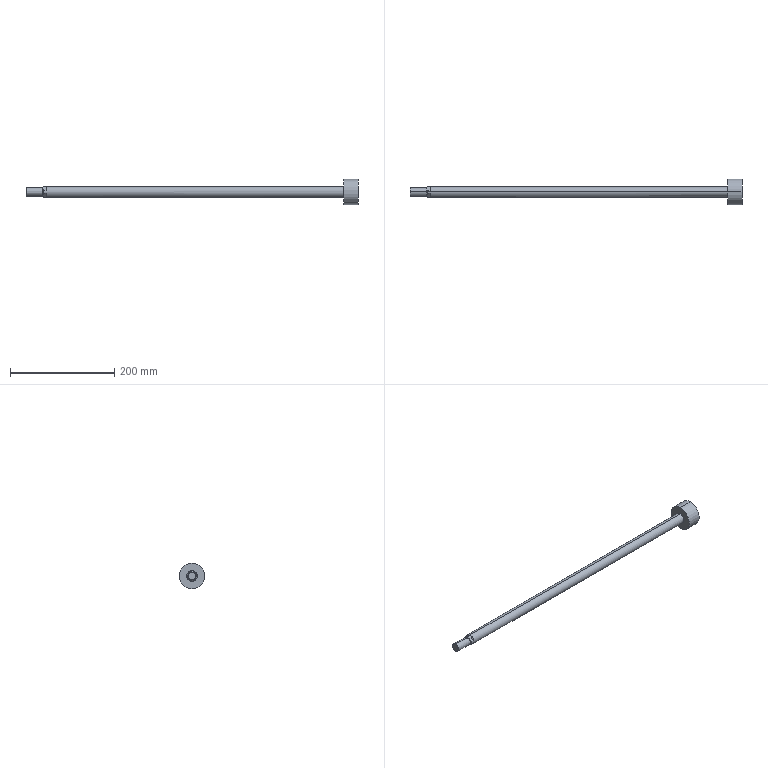Part | NX | features BREP 1 | 1 solid | 21 faces | box 635.5 x 49.1 x 49.1 mm | volume 238288 mm3 | plane 11 | cylinder 6 | cone 4 | commonest cylinder face diameters 16 x2 20 x2 49.1 x2
STEP:
#1=CARTESIAN_POINT('',(539.5,0.,10.));
#2=VERTEX_POINT('',#1);
#3=CARTESIAN_POINT('',(539.5,0.,-10.));
#4=VERTEX_POINT('',#3);
#5=CARTESIAN_POINT('',(539.5,0.,0.));
#6=DIRECTION('',(-1.,0.,0.));
#7=DIRECTION('',(0.,0.,1.));
#8=AXIS2_PLACEMENT_3D('',#5,#6,#7);
#9=CIRCLE('',#8,10.);
#10=EDGE_CURVE('',#2,#4,#9,.T.);
#11=ORIENTED_EDGE('',*,*,#10,.T.);
#12=CARTESIAN_POINT('',(-35.,0.,-10.));
#13=VERTEX_POINT('',#12);
#14=CARTESIAN_POINT('',(566.5,0.,-10.));
#15=DIRECTION('',(-1.,0.,0.));
#16=VECTOR('',#15,1000.);
#17=LINE('',#14,#16);
#18=EDGE_CURVE('',#13,#4,#17,.F.);
#19=ORIENTED_EDGE('',*,*,#18,.F.);
#20=CARTESIAN_POINT('',(-35.,2.285,-9.735));
#21=VERTEX_POINT('',#20);
#22=CARTESIAN_POINT('',(-35.,0.,0.));
#23=DIRECTION('',(1.,0.,0.));
#24=DIRECTION('',(0.,0.,1.));
#25=AXIS2_PLACEMENT_3D('',#22,#23,#24);
#26=CIRCLE('',#25,10.);
#27=EDGE_CURVE('',#13,#21,#26,.T.);
#28=ORIENTED_EDGE('',*,*,#27,.T.);
#29=CARTESIAN_POINT('',(-30.5,2.285,-9.735));
#30=VERTEX_POINT('',#29);
#31=CARTESIAN_POINT('',(566.5,2.285,-9.735));
#32=DIRECTION('',(1.,0.,0.));
#33=VECTOR('',#32,1000.);
#34=LINE('',#31,#33);
#35=EDGE_CURVE('',#21,#30,#34,.T.);
#36=ORIENTED_EDGE('',*,*,#35,.T.);
#37=CARTESIAN_POINT('',(-30.5,9.735,-2.285));
#38=VERTEX_POINT('',#37);
#39=CARTESIAN_POINT('',(-30.5,2.285,-9.735));
#40=CARTESIAN_POINT('',(-28.444,6.084,-8.844));
#41=CARTESIAN_POINT('',(-28.444,8.844,-6.084));
#42=CARTESIAN_POINT('',(-30.5,9.735,-2.285));
#43=(BOUNDED_CURVE()B_SPLINE_CURVE(3,(#39,#40,#41,#42),.UNSPECIFIED.,.F.,.F.)B_SPLINE_CURVE_WITH_KNOTS((4,4),(2.587,3.696),.UNSPECIFIED.)CURVE()GEOMETRIC_REPRESENTATION_ITEM()RATIONAL_B_SPLINE_CURVE((1.,0.9,0.9,1.))REPRESENTATION_ITEM(''));
#44=EDGE_CURVE('',#30,#38,#43,.T.);
#45=ORIENTED_EDGE('',*,*,#44,.T.);
#46=CARTESIAN_POINT('',(-35.,9.735,-2.285));
#47=VERTEX_POINT('',#46);
#48=CARTESIAN_POINT('',(566.5,9.735,-2.285));
#49=DIRECTION('',(-1.,0.,0.));
#50=VECTOR('',#49,1000.);
#51=LINE('',#48,#50);
#52=EDGE_CURVE('',#38,#47,#51,.T.);
#53=ORIENTED_EDGE('',*,*,#52,.T.);
#54=CARTESIAN_POINT('',(-35.,9.735,2.285));
#55=VERTEX_POINT('',#54);
#56=CARTESIAN_POINT('',(-35.,0.,0.));
#57=DIRECTION('',(1.,0.,0.));
#58=DIRECTION('',(0.,0.,1.));
#59=AXIS2_PLACEMENT_3D('',#56,#57,#58);
#60=CIRCLE('',#59,10.);
#61=EDGE_CURVE('',#47,#55,#60,.T.);
#62=ORIENTED_EDGE('',*,*,#61,.T.);
#63=CARTESIAN_POINT('',(-30.5,9.735,2.285));
#64=VERTEX_POINT('',#63);
#65=CARTESIAN_POINT('',(566.5,9.735,2.285));
#66=DIRECTION('',(1.,0.,0.));
#67=VECTOR('',#66,1000.);
#68=LINE('',#65,#67);
#69=EDGE_CURVE('',#55,#64,#68,.T.);
#70=ORIENTED_EDGE('',*,*,#69,.T.);
#71=CARTESIAN_POINT('',(-30.5,2.285,9.735));
#72=VERTEX_POINT('',#71);
#73=CARTESIAN_POINT('',(-30.5,9.735,2.285));
#74=CARTESIAN_POINT('',(-28.444,8.844,6.084));
#75=CARTESIAN_POINT('',(-28.444,6.084,8.844));
#76=CARTESIAN_POINT('',(-30.5,2.285,9.735));
#77=(BOUNDED_CURVE()B_SPLINE_CURVE(3,(#73,#74,#75,#76),.UNSPECIFIED.,.F.,.F.)B_SPLINE_CURVE_WITH_KNOTS((4,4),(2.587,3.696),.UNSPECIFIED.)CURVE()GEOMETRIC_REPRESENTATION_ITEM()RATIONAL_B_SPLINE_CURVE((1.,0.9,0.9,1.))REPRESENTATION_ITEM(''));
#78=EDGE_CURVE('',#64,#72,#77,.T.);
#79=ORIENTED_EDGE('',*,*,#78,.T.);
#80=CARTESIAN_POINT('',(-35.,2.285,9.735));
#81=VERTEX_POINT('',#80);
#82=CARTESIAN_POINT('',(566.5,2.285,9.735));
#83=DIRECTION('',(-1.,0.,0.));
#84=VECTOR('',#83,1000.);
#85=LINE('',#82,#84);
#86=EDGE_CURVE('',#72,#81,#85,.T.);
#87=ORIENTED_EDGE('',*,*,#86,.T.);
#88=CARTESIAN_POINT('',(-35.,0.,10.));
#89=VERTEX_POINT('',#88);
#90=CARTESIAN_POINT('',(-35.,0.,0.));
#91=DIRECTION('',(1.,0.,0.));
#92=DIRECTION('',(0.,0.,1.));
#93=AXIS2_PLACEMENT_3D('',#90,#91,#92);
#94=CIRCLE('',#93,10.);
#95=EDGE_CURVE('',#81,#89,#94,.T.);
#96=ORIENTED_EDGE('',*,*,#95,.T.);
#97=CARTESIAN_POINT('',(566.5,0.,10.));
#98=DIRECTION('',(-1.,0.,0.));
#99=VECTOR('',#98,1000.);
#100=LINE('',#97,#99);
#101=EDGE_CURVE('',#89,#2,#100,.F.);
#102=ORIENTED_EDGE('',*,*,#101,.T.);
#103=EDGE_LOOP('',(#11,#19,#28,#36,#45,#53,#62,#70,#79,#87,#96,#102));
#104=FACE_BOUND('',#103,.T.);
#105=CARTESIAN_POINT('',(566.5,0.,0.));
#106=DIRECTION('',(-1.,0.,0.));
#107=DIRECTION('',(0.,0.,1.));
#108=AXIS2_PLACEMENT_3D('',#105,#106,#107);
#109=CYLINDRICAL_SURFACE('',#108,10.);
#110=ADVANCED_FACE('',(#104),#109,.T.);
#111=CARTESIAN_POINT('',(-37.,0.,-8.));
#112=VERTEX_POINT('',#111);
#113=CARTESIAN_POINT('',(-37.,0.,8.));
#114=VERTEX_POINT('',#113);
#115=CARTESIAN_POINT('',(-37.,0.,0.));
#116=DIRECTION('',(1.,0.,0.));
#117=DIRECTION('',(0.,0.,-1.));
#118=AXIS2_PLACEMENT_3D('',#115,#116,#117);
#119=CIRCLE('',#118,8.);
#120=EDGE_CURVE('',#112,#114,#119,.T.);
#121=ORIENTED_EDGE('',*,*,#120,.T.);
#122=CARTESIAN_POINT('',(-35.,0.,10.));
#123=DIRECTION('',(0.7071,0.,0.7071));
#124=VECTOR('',#123,1000.);
#125=LINE('',#122,#124);
#126=EDGE_CURVE('',#114,#89,#125,.T.);
#127=ORIENTED_EDGE('',*,*,#126,.T.);
#128=ORIENTED_EDGE('',*,*,#95,.F.);
#129=CARTESIAN_POINT('',(-35.,9.735,2.285));
#130=CARTESIAN_POINT('',(-35.469,9.106,2.915));
#131=CARTESIAN_POINT('',(-35.982,8.278,3.743));
#132=CARTESIAN_POINT('',(-36.426,6.984,5.037));
#133=CARTESIAN_POINT('',(-36.537,6.009,6.011));
#134=CARTESIAN_POINT('',(-36.427,5.037,6.984));
#135=CARTESIAN_POINT('',(-36.089,4.056,7.965));
#136=CARTESIAN_POINT('',(-35.654,3.227,8.794));
#137=CARTESIAN_POINT('',(-35.236,2.602,9.419));
#138=CARTESIAN_POINT('',(-35.,2.285,9.735));
#139=B_SPLINE_CURVE_WITH_KNOTS('',3,(#129,#130,#131,#132,#133,#134,#135,#136,#137,#138),.UNSPECIFIED.,.F.,.F.,(4,1,1,1,1,1,1,4),(0.,0.25,0.375,0.5,0.625,0.75,0.875,1.),.UNSPECIFIED.);
#140=EDGE_CURVE('',#81,#55,#139,.F.);
#141=ORIENTED_EDGE('',*,*,#140,.T.);
#142=ORIENTED_EDGE('',*,*,#61,.F.);
#143=CARTESIAN_POINT('',(-35.,2.285,-9.735));
#144=CARTESIAN_POINT('',(-35.469,2.915,-9.106));
#145=CARTESIAN_POINT('',(-35.982,3.743,-8.278));
#146=CARTESIAN_POINT('',(-36.426,5.037,-6.984));
#147=CARTESIAN_POINT('',(-36.537,6.011,-6.009));
#148=CARTESIAN_POINT('',(-36.427,6.984,-5.037));
#149=CARTESIAN_POINT('',(-36.089,7.965,-4.056));
#150=CARTESIAN_POINT('',(-35.654,8.794,-3.227));
#151=CARTESIAN_POINT('',(-35.236,9.419,-2.602));
#152=CARTESIAN_POINT('',(-35.,9.735,-2.285));
#153=B_SPLINE_CURVE_WITH_KNOTS('',3,(#143,#144,#145,#146,#147,#148,#149,#150,#151,#152),.UNSPECIFIED.,.F.,.F.,(4,1,1,1,1,1,1,4),(0.,0.25,0.375,0.5,0.625,0.75,0.875,1.),.UNSPECIFIED.);
#154=EDGE_CURVE('',#47,#21,#153,.F.);
#155=ORIENTED_EDGE('',*,*,#154,.T.);
#156=ORIENTED_EDGE('',*,*,#27,.F.);
#157=CARTESIAN_POINT('',(-35.,0.,-10.));
#158=DIRECTION('',(0.7071,0.,-0.7071));
#159=VECTOR('',#158,1000.);
#160=LINE('',#157,#159);
#161=EDGE_CURVE('',#112,#13,#160,.T.);
#162=ORIENTED_EDGE('',*,*,#161,.F.);
#163=EDGE_LOOP('',(#121,#127,#128,#141,#142,#155,#156,#162));
#164=FACE_BOUND('',#163,.T.);
#165=CARTESIAN_POINT('',(-35.,0.,0.));
#166=DIRECTION('',(1.,0.,0.));
#167=DIRECTION('',(0.,0.,-1.));
#168=AXIS2_PLACEMENT_3D('',#165,#166,#167);
#169=CONICAL_SURFACE('',#168,10.,0.7854);
#170=ADVANCED_FACE('',(#164),#169,.T.);
#171=ORIENTED_EDGE('',*,*,#120,.F.);
#172=CARTESIAN_POINT('',(-68.08,0.,-8.));
#173=VERTEX_POINT('',#172);
#174=CARTESIAN_POINT('',(566.5,0.,-8.));
#175=DIRECTION('',(-1.,0.,0.));
#176=VECTOR('',#175,1000.);
#177=LINE('',#174,#176);
#178=EDGE_CURVE('',#173,#112,#177,.F.);
#179=ORIENTED_EDGE('',*,*,#178,.F.);
#180=CARTESIAN_POINT('',(-68.08,0.,8.));
#181=VERTEX_POINT('',#180);
#182=CARTESIAN_POINT('',(-68.08,0.,0.));
#183=DIRECTION('',(1.,0.,0.));
#184=DIRECTION('',(0.,0.,1.));
#185=AXIS2_PLACEMENT_3D('',#182,#183,#184);
#186=CIRCLE('',#185,8.);
#187=EDGE_CURVE('',#173,#181,#186,.T.);
#188=ORIENTED_EDGE('',*,*,#187,.T.);
#189=CARTESIAN_POINT('',(566.5,0.,8.));
#190=DIRECTION('',(-1.,0.,0.));
#191=VECTOR('',#190,1000.);
#192=LINE('',#189,#191);
#193=EDGE_CURVE('',#181,#114,#192,.F.);
#194=ORIENTED_EDGE('',*,*,#193,.T.);
#195=EDGE_LOOP('',(#171,#179,#188,#194));
#196=FACE_BOUND('',#195,.T.);
#197=CARTESIAN_POINT('',(566.5,0.,0.));
#198=DIRECTION('',(-1.,0.,0.));
#199=DIRECTION('',(0.,0.,1.));
#200=AXIS2_PLACEMENT_3D('',#197,#198,#199);
#201=CYLINDRICAL_SURFACE('',#200,8.);
#202=ADVANCED_FACE('',(#196),#201,.T.);
#203=CARTESIAN_POINT('',(566.5,0.,24.55));
#204=VERTEX_POINT('',#203);
#205=CARTESIAN_POINT('',(566.5,0.,-24.55));
#206=VERTEX_POINT('',#205);
#207=CARTESIAN_POINT('',(566.5,0.,0.));
#208=DIRECTION('',(-1.,0.,0.));
#209=DIRECTION('',(0.,0.,1.));
#210=AXIS2_PLACEMENT_3D('',#207,#208,#209);
#211=CIRCLE('',#210,24.55);
#212=EDGE_CURVE('',#204,#206,#211,.T.);
#213=ORIENTED_EDGE('',*,*,#212,.T.);
#214=CARTESIAN_POINT('',(539.5,0.,-24.55));
#215=VERTEX_POINT('',#214);
#216=CARTESIAN_POINT('',(566.5,0.,-24.55));
#217=DIRECTION('',(-1.,0.,0.));
#218=VECTOR('',#217,1000.);
#219=LINE('',#216,#218);
#220=EDGE_CURVE('',#215,#206,#219,.F.);
#221=ORIENTED_EDGE('',*,*,#220,.F.);
#222=CARTESIAN_POINT('',(539.5,0.,24.55));
#223=VERTEX_POINT('',#222);
#224=CARTESIAN_POINT('',(539.5,0.,0.));
#225=DIRECTION('',(1.,0.,0.));
#226=DIRECTION('',(0.,0.,1.));
#227=AXIS2_PLACEMENT_3D('',#224,#225,#226);
#228=CIRCLE('',#227,24.55);
#229=EDGE_CURVE('',#215,#223,#228,.T.);
#230=ORIENTED_EDGE('',*,*,#229,.T.);
#231=CARTESIAN_POINT('',(566.5,0.,24.55));
#232=DIRECTION('',(-1.,0.,0.));
#233=VECTOR('',#232,1000.);
#234=LINE('',#231,#233);
#235=EDGE_CURVE('',#223,#204,#234,.F.);
#236=ORIENTED_EDGE('',*,*,#235,.T.);
#237=EDGE_LOOP('',(#213,#221,#230,#236));
#238=FACE_BOUND('',#237,.T.);
#239=CARTESIAN_POINT('',(566.5,0.,0.));
#240=DIRECTION('',(-1.,0.,0.));
#241=DIRECTION('',(0.,0.,1.));
#242=AXIS2_PLACEMENT_3D('',#239,#240,#241);
#243=CYLINDRICAL_SURFACE('',#242,24.55);
#244=ADVANCED_FACE('',(#238),#243,.T.);
#245=CARTESIAN_POINT('',(-69.,0.,-7.08));
#246=VERTEX_POINT('',#245);
#247=CARTESIAN_POINT('',(-69.,0.,7.08));
#248=VERTEX_POINT('',#247);
#249=CARTESIAN_POINT('',(-69.,0.,0.));
#250=DIRECTION('',(1.,0.,0.));
#251=DIRECTION('',(0.,0.,-1.));
#252=AXIS2_PLACEMENT_3D('',#249,#250,#251);
#253=CIRCLE('',#252,7.08);
#254=EDGE_CURVE('',#246,#248,#253,.T.);
#255=ORIENTED_EDGE('',*,*,#254,.T.);
#256=CARTESIAN_POINT('',(-68.08,0.,8.));
#257=DIRECTION('',(0.7071,0.,0.7071));
#258=VECTOR('',#257,1000.);
#259=LINE('',#256,#258);
#260=EDGE_CURVE('',#248,#181,#259,.T.);
#261=ORIENTED_EDGE('',*,*,#260,.T.);
#262=ORIENTED_EDGE('',*,*,#187,.F.);
#263=CARTESIAN_POINT('',(-68.08,0.,-8.));
#264=DIRECTION('',(0.7071,0.,-0.7071));
#265=VECTOR('',#264,1000.);
#266=LINE('',#263,#265);
#267=EDGE_CURVE('',#246,#173,#266,.T.);
#268=ORIENTED_EDGE('',*,*,#267,.F.);
#269=EDGE_LOOP('',(#255,#261,#262,#268));
#270=FACE_BOUND('',#269,.T.);
#271=CARTESIAN_POINT('',(-68.08,0.,0.));
#272=DIRECTION('',(1.,0.,0.));
#273=DIRECTION('',(0.,0.,-1.));
#274=AXIS2_PLACEMENT_3D('',#271,#272,#273);
#275=CONICAL_SURFACE('',#274,8.,0.7854);
#276=ADVANCED_FACE('',(#270),#275,.T.);
#277=ORIENTED_EDGE('',*,*,#18,.T.);
#278=CARTESIAN_POINT('',(539.5,0.,0.));
#279=DIRECTION('',(-1.,0.,0.));
#280=DIRECTION('',(0.,0.,1.));
#281=AXIS2_PLACEMENT_3D('',#278,#279,#280);
#282=CIRCLE('',#281,10.);
#283=EDGE_CURVE('',#4,#2,#282,.T.);
#284=ORIENTED_EDGE('',*,*,#283,.T.);
#285=ORIENTED_EDGE('',*,*,#101,.F.);
#286=CARTESIAN_POINT('',(-35.,-2.285,9.735));
#287=VERTEX_POINT('',#286);
#288=CARTESIAN_POINT('',(-35.,0.,0.));
#289=DIRECTION('',(1.,0.,0.));
#290=DIRECTION('',(0.,0.,1.));
#291=AXIS2_PLACEMENT_3D('',#288,#289,#290);
#292=CIRCLE('',#291,10.);
#293=EDGE_CURVE('',#89,#287,#292,.T.);
#294=ORIENTED_EDGE('',*,*,#293,.T.);
#295=CARTESIAN_POINT('',(-30.5,-2.285,9.735));
#296=VERTEX_POINT('',#295);
#297=CARTESIAN_POINT('',(566.5,-2.285,9.735));
#298=DIRECTION('',(1.,0.,0.));
#299=VECTOR('',#298,1000.);
#300=LINE('',#297,#299);
#301=EDGE_CURVE('',#287,#296,#300,.T.);
#302=ORIENTED_EDGE('',*,*,#301,.T.);
#303=CARTESIAN_POINT('',(-30.5,-9.735,2.285));
#304=VERTEX_POINT('',#303);
#305=CARTESIAN_POINT('',(-30.5,-2.285,9.735));
#306=CARTESIAN_POINT('',(-28.444,-6.084,8.844));
#307=CARTESIAN_POINT('',(-28.444,-8.844,6.084));
#308=CARTESIAN_POINT('',(-30.5,-9.735,2.285));
#309=(BOUNDED_CURVE()B_SPLINE_CURVE(3,(#305,#306,#307,#308),.UNSPECIFIED.,.F.,.F.)B_SPLINE_CURVE_WITH_KNOTS((4,4),(2.587,3.696),.UNSPECIFIED.)CURVE()GEOMETRIC_REPRESENTATION_ITEM()RATIONAL_B_SPLINE_CURVE((1.,0.9,0.9,1.))REPRESENTATION_ITEM(''));
#310=EDGE_CURVE('',#296,#304,#309,.T.);
#311=ORIENTED_EDGE('',*,*,#310,.T.);
#312=CARTESIAN_POINT('',(-35.,-9.735,2.285));
#313=VERTEX_POINT('',#312);
#314=CARTESIAN_POINT('',(566.5,-9.735,2.285));
#315=DIRECTION('',(-1.,0.,0.));
#316=VECTOR('',#315,1000.);
#317=LINE('',#314,#316);
#318=EDGE_CURVE('',#304,#313,#317,.T.);
#319=ORIENTED_EDGE('',*,*,#318,.T.);
#320=CARTESIAN_POINT('',(-35.,-9.735,-2.285));
#321=VERTEX_POINT('',#320);
#322=CARTESIAN_POINT('',(-35.,0.,0.));
#323=DIRECTION('',(1.,0.,0.));
#324=DIRECTION('',(0.,0.,1.));
#325=AXIS2_PLACEMENT_3D('',#322,#323,#324);
#326=CIRCLE('',#325,10.);
#327=EDGE_CURVE('',#313,#321,#326,.T.);
#328=ORIENTED_EDGE('',*,*,#327,.T.);
#329=CARTESIAN_POINT('',(-30.5,-9.735,-2.285));
#330=VERTEX_POINT('',#329);
#331=CARTESIAN_POINT('',(566.5,-9.735,-2.285));
#332=DIRECTION('',(1.,0.,0.));
#333=VECTOR('',#332,1000.);
#334=LINE('',#331,#333);
#335=EDGE_CURVE('',#321,#330,#334,.T.);
#336=ORIENTED_EDGE('',*,*,#335,.T.);
#337=CARTESIAN_POINT('',(-30.5,-2.285,-9.735));
#338=VERTEX_POINT('',#337);
#339=CARTESIAN_POINT('',(-30.5,-9.735,-2.285));
#340=CARTESIAN_POINT('',(-28.444,-8.844,-6.084));
#341=CARTESIAN_POINT('',(-28.444,-6.084,-8.844));
#342=CARTESIAN_POINT('',(-30.5,-2.285,-9.735));
#343=(BOUNDED_CURVE()B_SPLINE_CURVE(3,(#339,#340,#341,#342),.UNSPECIFIED.,.F.,.F.)B_SPLINE_CURVE_WITH_KNOTS((4,4),(2.587,3.696),.UNSPECIFIED.)CURVE()GEOMETRIC_REPRESENTATION_ITEM()RATIONAL_B_SPLINE_CURVE((1.,0.9,0.9,1.))REPRESENTATION_ITEM(''));
#344=EDGE_CURVE('',#330,#338,#343,.T.);
#345=ORIENTED_EDGE('',*,*,#344,.T.);
#346=CARTESIAN_POINT('',(-35.,-2.285,-9.735));
#347=VERTEX_POINT('',#346);
#348=CARTESIAN_POINT('',(566.5,-2.285,-9.735));
#349=DIRECTION('',(-1.,0.,0.));
#350=VECTOR('',#349,1000.);
#351=LINE('',#348,#350);
#352=EDGE_CURVE('',#338,#347,#351,.T.);
#353=ORIENTED_EDGE('',*,*,#352,.T.);
#354=CARTESIAN_POINT('',(-35.,0.,0.));
#355=DIRECTION('',(1.,0.,0.));
#356=DIRECTION('',(0.,0.,1.));
#357=AXIS2_PLACEMENT_3D('',#354,#355,#356);
#358=CIRCLE('',#357,10.);
#359=EDGE_CURVE('',#347,#13,#358,.T.);
#360=ORIENTED_EDGE('',*,*,#359,.T.);
#361=EDGE_LOOP('',(#277,#284,#285,#294,#302,#311,#319,#328,#336,#345,#353,#360));
#362=FACE_BOUND('',#361,.T.);
#363=CARTESIAN_POINT('',(566.5,0.,0.));
#364=DIRECTION('',(-1.,0.,0.));
#365=DIRECTION('',(0.,0.,1.));
#366=AXIS2_PLACEMENT_3D('',#363,#364,#365);
#367=CYLINDRICAL_SURFACE('',#366,10.);
#368=ADVANCED_FACE('',(#362),#367,.T.);
#369=ORIENTED_EDGE('',*,*,#344,.F.);
#370=CARTESIAN_POINT('',(-30.5,-9.735,-2.285));
#371=DIRECTION('',(0.,0.7071,-0.7071));
#372=VECTOR('',#371,1000.);
#373=LINE('',#370,#372);
#374=EDGE_CURVE('',#330,#338,#373,.T.);
#375=ORIENTED_EDGE('',*,*,#374,.T.);
#376=EDGE_LOOP('',(#369,#375));
#377=FACE_BOUND('',#376,.T.);
#378=CARTESIAN_POINT('',(-29.,-13.081,-1.061));
#379=DIRECTION('',(-0.7071,-0.5,-0.5));
#380=DIRECTION('',(-0.5774,0.,0.8165));
#381=AXIS2_PLACEMENT_3D('',#378,#379,#380);
#382=PLANE('',#381);
#383=ADVANCED_FACE('',(#377),#382,.T.);
#384=ORIENTED_EDGE('',*,*,#335,.F.);
#385=CARTESIAN_POINT('',(-35.,-9.735,-2.285));
#386=CARTESIAN_POINT('',(-35.236,-9.419,-2.602));
#387=CARTESIAN_POINT('',(-35.654,-8.791,-3.229));
#388=CARTESIAN_POINT('',(-36.087,-7.974,-4.047));
#389=CARTESIAN_POINT('',(-36.435,-6.949,-5.071));
#390=CARTESIAN_POINT('',(-36.533,-6.011,-6.01));
#391=CARTESIAN_POINT('',(-36.435,-5.074,-6.947));
#392=CARTESIAN_POINT('',(-36.088,-4.047,-7.973));
#393=CARTESIAN_POINT('',(-35.655,-3.231,-8.79));
#394=CARTESIAN_POINT('',(-35.236,-2.602,-9.419));
#395=CARTESIAN_POINT('',(-35.,-2.285,-9.735));
#396=B_SPLINE_CURVE_WITH_KNOTS('',3,(#385,#386,#387,#388,#389,#390,#391,#392,#393,#394,#395),.UNSPECIFIED.,.F.,.F.,(4,1,1,1,1,1,1,1,4),(0.,0.125,0.25,0.375,0.5,0.625,0.75,0.875,1.),.UNSPECIFIED.);
#397=EDGE_CURVE('',#321,#347,#396,.T.);
#398=ORIENTED_EDGE('',*,*,#397,.T.);
#399=ORIENTED_EDGE('',*,*,#352,.F.);
#400=ORIENTED_EDGE('',*,*,#374,.F.);
#401=EDGE_LOOP('',(#384,#398,#399,#400));
#402=FACE_BOUND('',#401,.T.);
#403=CARTESIAN_POINT('',(-30.5,-12.021,0.));
#404=DIRECTION('',(0.,-0.7071,-0.7071));
#405=DIRECTION('',(0.,0.7071,-0.7071));
#406=AXIS2_PLACEMENT_3D('',#403,#404,#405);
#407=PLANE('',#406);
#408=ADVANCED_FACE('',(#402),#407,.T.);
#409=ORIENTED_EDGE('',*,*,#126,.F.);
#410=CARTESIAN_POINT('',(-37.,0.,0.));
#411=DIRECTION('',(1.,0.,0.));
#412=DIRECTION('',(0.,0.,-1.));
#413=AXIS2_PLACEMENT_3D('',#410,#411,#412);
#414=CIRCLE('',#413,8.);
#415=EDGE_CURVE('',#114,#112,#414,.T.);
#416=ORIENTED_EDGE('',*,*,#415,.T.);
#417=ORIENTED_EDGE('',*,*,#161,.T.);
#418=ORIENTED_EDGE('',*,*,#359,.F.);
#419=ORIENTED_EDGE('',*,*,#397,.F.);
#420=ORIENTED_EDGE('',*,*,#327,.F.);
#421=CARTESIAN_POINT('',(-35.,-2.285,9.735));
#422=CARTESIAN_POINT('',(-35.469,-2.915,9.106));
#423=CARTESIAN_POINT('',(-35.982,-3.743,8.278));
#424=CARTESIAN_POINT('',(-36.426,-5.037,6.984));
#425=CARTESIAN_POINT('',(-36.537,-6.011,6.009));
#426=CARTESIAN_POINT('',(-36.427,-6.984,5.037));
#427=CARTESIAN_POINT('',(-36.089,-7.965,4.056));
#428=CARTESIAN_POINT('',(-35.654,-8.794,3.227));
#429=CARTESIAN_POINT('',(-35.236,-9.419,2.602));
#430=CARTESIAN_POINT('',(-35.,-9.735,2.285));
#431=B_SPLINE_CURVE_WITH_KNOTS('',3,(#421,#422,#423,#424,#425,#426,#427,#428,#429,#430),.UNSPECIFIED.,.F.,.F.,(4,1,1,1,1,1,1,4),(0.,0.25,0.375,0.5,0.625,0.75,0.875,1.),.UNSPECIFIED.);
#432=EDGE_CURVE('',#313,#287,#431,.F.);
#433=ORIENTED_EDGE('',*,*,#432,.T.);
#434=ORIENTED_EDGE('',*,*,#293,.F.);
#435=EDGE_LOOP('',(#409,#416,#417,#418,#419,#420,#433,#434));
#436=FACE_BOUND('',#435,.T.);
#437=CARTESIAN_POINT('',(-35.,0.,0.));
#438=DIRECTION('',(1.,0.,0.));
#439=DIRECTION('',(0.,0.,-1.));
#440=AXIS2_PLACEMENT_3D('',#437,#438,#439);
#441=CONICAL_SURFACE('',#440,10.,0.7854);
#442=ADVANCED_FACE('',(#436),#441,.T.);
#443=ORIENTED_EDGE('',*,*,#301,.F.);
#444=ORIENTED_EDGE('',*,*,#432,.F.);
#445=ORIENTED_EDGE('',*,*,#318,.F.);
#446=CARTESIAN_POINT('',(-30.5,0.,12.021));
#447=DIRECTION('',(0.,0.7071,0.7071));
#448=VECTOR('',#447,1000.);
#449=LINE('',#446,#448);
#450=EDGE_CURVE('',#304,#296,#449,.T.);
#451=ORIENTED_EDGE('',*,*,#450,.T.);
#452=EDGE_LOOP('',(#443,#444,#445,#451));
#453=FACE_BOUND('',#452,.T.);
#454=CARTESIAN_POINT('',(-30.5,0.,12.021));
#455=DIRECTION('',(0.,-0.7071,0.7071));
#456=DIRECTION('',(-1.,0.,0.));
#457=AXIS2_PLACEMENT_3D('',#454,#455,#456);
#458=PLANE('',#457);
#459=ADVANCED_FACE('',(#453),#458,.T.);
#460=ORIENTED_EDGE('',*,*,#310,.F.);
#461=ORIENTED_EDGE('',*,*,#450,.F.);
#462=EDGE_LOOP('',(#460,#461));
#463=FACE_BOUND('',#462,.T.);
#464=CARTESIAN_POINT('',(-29.,-1.061,13.081));
#465=DIRECTION('',(-0.7071,-0.5,0.5));
#466=DIRECTION('',(-0.5774,0.8165,0.));
#467=AXIS2_PLACEMENT_3D('',#464,#465,#466);
#468=PLANE('',#467);
#469=ADVANCED_FACE('',(#463),#468,.T.);
#470=ORIENTED_EDGE('',*,*,#69,.F.);
#471=ORIENTED_EDGE('',*,*,#140,.F.);
#472=ORIENTED_EDGE('',*,*,#86,.F.);
#473=CARTESIAN_POINT('',(-30.5,0.,12.021));
#474=DIRECTION('',(0.,0.7071,-0.7071));
#475=VECTOR('',#474,1000.);
#476=LINE('',#473,#475);
#477=EDGE_CURVE('',#72,#64,#476,.T.);
#478=ORIENTED_EDGE('',*,*,#477,.T.);
#479=EDGE_LOOP('',(#470,#471,#472,#478));
#480=FACE_BOUND('',#479,.T.);
#481=CARTESIAN_POINT('',(-71.7,0.,12.021));
#482=DIRECTION('',(0.,0.7071,0.7071));
#483=DIRECTION('',(1.,0.,0.));
#484=AXIS2_PLACEMENT_3D('',#481,#482,#483);
#485=PLANE('',#484);
#486=ADVANCED_FACE('',(#480),#485,.T.);
#487=ORIENTED_EDGE('',*,*,#78,.F.);
#488=ORIENTED_EDGE('',*,*,#477,.F.);
#489=EDGE_LOOP('',(#487,#488));
#490=FACE_BOUND('',#489,.T.);
#491=CARTESIAN_POINT('',(-30.5,0.,12.021));
#492=DIRECTION('',(-0.7071,0.5,0.5));
#493=DIRECTION('',(0.5774,0.8165,0.));
#494=AXIS2_PLACEMENT_3D('',#491,#492,#493);
#495=PLANE('',#494);
#496=ADVANCED_FACE('',(#490),#495,.T.);
#497=ORIENTED_EDGE('',*,*,#35,.F.);
#498=ORIENTED_EDGE('',*,*,#154,.F.);
#499=ORIENTED_EDGE('',*,*,#52,.F.);
#500=CARTESIAN_POINT('',(-30.5,12.021,0.));
#501=DIRECTION('',(0.,-0.7071,-0.7071));
#502=VECTOR('',#501,1000.);
#503=LINE('',#500,#502);
#504=EDGE_CURVE('',#38,#30,#503,.T.);
#505=ORIENTED_EDGE('',*,*,#504,.T.);
#506=EDGE_LOOP('',(#497,#498,#499,#505));
#507=FACE_BOUND('',#506,.T.);
#508=CARTESIAN_POINT('',(-71.7,12.021,0.));
#509=DIRECTION('',(0.,0.7071,-0.7071));
#510=DIRECTION('',(-1.,0.,0.));
#511=AXIS2_PLACEMENT_3D('',#508,#509,#510);
#512=PLANE('',#511);
#513=ADVANCED_FACE('',(#507),#512,.T.);
#514=ORIENTED_EDGE('',*,*,#44,.F.);
#515=ORIENTED_EDGE('',*,*,#504,.F.);
#516=EDGE_LOOP('',(#514,#515));
#517=FACE_BOUND('',#516,.T.);
#518=CARTESIAN_POINT('',(-30.5,12.021,0.));
#519=DIRECTION('',(-0.7071,0.5,-0.5));
#520=DIRECTION('',(-0.5774,0.,0.8165));
#521=AXIS2_PLACEMENT_3D('',#518,#519,#520);
#522=PLANE('',#521);
#523=ADVANCED_FACE('',(#517),#522,.T.);
#524=CARTESIAN_POINT('',(539.5,0.,0.));
#525=DIRECTION('',(1.,0.,0.));
#526=DIRECTION('',(0.,0.,1.));
#527=AXIS2_PLACEMENT_3D('',#524,#525,#526);
#528=CIRCLE('',#527,24.55);
#529=EDGE_CURVE('',#223,#215,#528,.T.);
#530=ORIENTED_EDGE('',*,*,#529,.F.);
#531=ORIENTED_EDGE('',*,*,#229,.F.);
#532=EDGE_LOOP('',(#530,#531));
#533=FACE_BOUND('',#532,.T.);
#534=ORIENTED_EDGE('',*,*,#10,.F.);
#535=ORIENTED_EDGE('',*,*,#283,.F.);
#536=EDGE_LOOP('',(#534,#535));
#537=FACE_BOUND('',#536,.T.);
#538=CARTESIAN_POINT('',(539.5,10.,0.));
#539=DIRECTION('',(1.,0.,0.));
#540=DIRECTION('',(0.,1.,0.));
#541=AXIS2_PLACEMENT_3D('',#538,#539,#540);
#542=PLANE('',#541);
#543=ADVANCED_FACE('',(#533,#537),#542,.F.);
#544=ORIENTED_EDGE('',*,*,#178,.T.);
#545=ORIENTED_EDGE('',*,*,#415,.F.);
#546=ORIENTED_EDGE('',*,*,#193,.F.);
#547=CARTESIAN_POINT('',(-68.08,0.,0.));
#548=DIRECTION('',(1.,0.,0.));
#549=DIRECTION('',(0.,0.,1.));
#550=AXIS2_PLACEMENT_3D('',#547,#548,#549);
#551=CIRCLE('',#550,8.);
#552=EDGE_CURVE('',#181,#173,#551,.T.);
#553=ORIENTED_EDGE('',*,*,#552,.T.);
#554=EDGE_LOOP('',(#544,#545,#546,#553));
#555=FACE_BOUND('',#554,.T.);
#556=CARTESIAN_POINT('',(566.5,0.,0.));
#557=DIRECTION('',(-1.,0.,0.));
#558=DIRECTION('',(0.,0.,1.));
#559=AXIS2_PLACEMENT_3D('',#556,#557,#558);
#560=CYLINDRICAL_SURFACE('',#559,8.);
#561=ADVANCED_FACE('',(#555),#560,.T.);
#562=ORIENTED_EDGE('',*,*,#220,.T.);
#563=CARTESIAN_POINT('',(566.5,0.,0.));
#564=DIRECTION('',(-1.,0.,0.));
#565=DIRECTION('',(0.,0.,1.));
#566=AXIS2_PLACEMENT_3D('',#563,#564,#565);
#567=CIRCLE('',#566,24.55);
#568=EDGE_CURVE('',#206,#204,#567,.T.);
#569=ORIENTED_EDGE('',*,*,#568,.T.);
#570=ORIENTED_EDGE('',*,*,#235,.F.);
#571=ORIENTED_EDGE('',*,*,#529,.T.);
#572=EDGE_LOOP('',(#562,#569,#570,#571));
#573=FACE_BOUND('',#572,.T.);
#574=CARTESIAN_POINT('',(566.5,0.,0.));
#575=DIRECTION('',(-1.,0.,0.));
#576=DIRECTION('',(0.,0.,1.));
#577=AXIS2_PLACEMENT_3D('',#574,#575,#576);
#578=CYLINDRICAL_SURFACE('',#577,24.55);
#579=ADVANCED_FACE('',(#573),#578,.T.);
#580=ORIENTED_EDGE('',*,*,#260,.F.);
#581=CARTESIAN_POINT('',(-69.,0.,0.));
#582=DIRECTION('',(1.,0.,0.));
#583=DIRECTION('',(0.,0.,-1.));
#584=AXIS2_PLACEMENT_3D('',#581,#582,#583);
#585=CIRCLE('',#584,7.08);
#586=EDGE_CURVE('',#248,#246,#585,.T.);
#587=ORIENTED_EDGE('',*,*,#586,.T.);
#588=ORIENTED_EDGE('',*,*,#267,.T.);
#589=ORIENTED_EDGE('',*,*,#552,.F.);
#590=EDGE_LOOP('',(#580,#587,#588,#589));
#591=FACE_BOUND('',#590,.T.);
#592=CARTESIAN_POINT('',(-68.08,0.,0.));
#593=DIRECTION('',(1.,0.,0.));
#594=DIRECTION('',(0.,0.,-1.));
#595=AXIS2_PLACEMENT_3D('',#592,#593,#594);
#596=CONICAL_SURFACE('',#595,8.,0.7854);
#597=ADVANCED_FACE('',(#591),#596,.T.);
#598=ORIENTED_EDGE('',*,*,#212,.F.);
#599=ORIENTED_EDGE('',*,*,#568,.F.);
#600=EDGE_LOOP('',(#598,#599));
#601=FACE_BOUND('',#600,.T.);
#602=CARTESIAN_POINT('',(566.5,24.55,0.));
#603=DIRECTION('',(-1.,0.,0.));
#604=DIRECTION('',(0.,0.,1.));
#605=AXIS2_PLACEMENT_3D('',#602,#603,#604);
#606=PLANE('',#605);
#607=ADVANCED_FACE('',(#601),#606,.F.);
#608=ORIENTED_EDGE('',*,*,#254,.F.);
#609=ORIENTED_EDGE('',*,*,#586,.F.);
#610=EDGE_LOOP('',(#608,#609));
#611=FACE_BOUND('',#610,.T.);
#612=CARTESIAN_POINT('',(-69.,0.,0.));
#613=DIRECTION('',(1.,0.,0.));
#614=DIRECTION('',(0.,1.,0.));
#615=AXIS2_PLACEMENT_3D('',#612,#613,#614);
#616=PLANE('',#615);
#617=ADVANCED_FACE('',(#611),#616,.F.);
#618=CLOSED_SHELL('',(#110,#170,#202,#244,#276,#368,#383,#408,#442,#459,#469,#486,#496,#513,#523,#543,#561,#579,#597,#607,#617));
#619=MANIFOLD_SOLID_BREP('',#618);
#620=(LENGTH_UNIT()NAMED_UNIT(*)SI_UNIT(.MILLI.,.METRE.));
#621=UNCERTAINTY_MEASURE_WITH_UNIT(LENGTH_MEASURE(0.0508),#620,'','');
#622=(NAMED_UNIT(*)PLANE_ANGLE_UNIT()SI_UNIT($,.RADIAN.));
#623=(NAMED_UNIT(*)SI_UNIT($,.STERADIAN.)SOLID_ANGLE_UNIT());
#624=(GEOMETRIC_REPRESENTATION_CONTEXT(3)GLOBAL_UNCERTAINTY_ASSIGNED_CONTEXT((#621))GLOBAL_UNIT_ASSIGNED_CONTEXT((#620,#622,#623))REPRESENTATION_CONTEXT('',''));
#625=ADVANCED_BREP_SHAPE_REPRESENTATION('',(#619),#624);